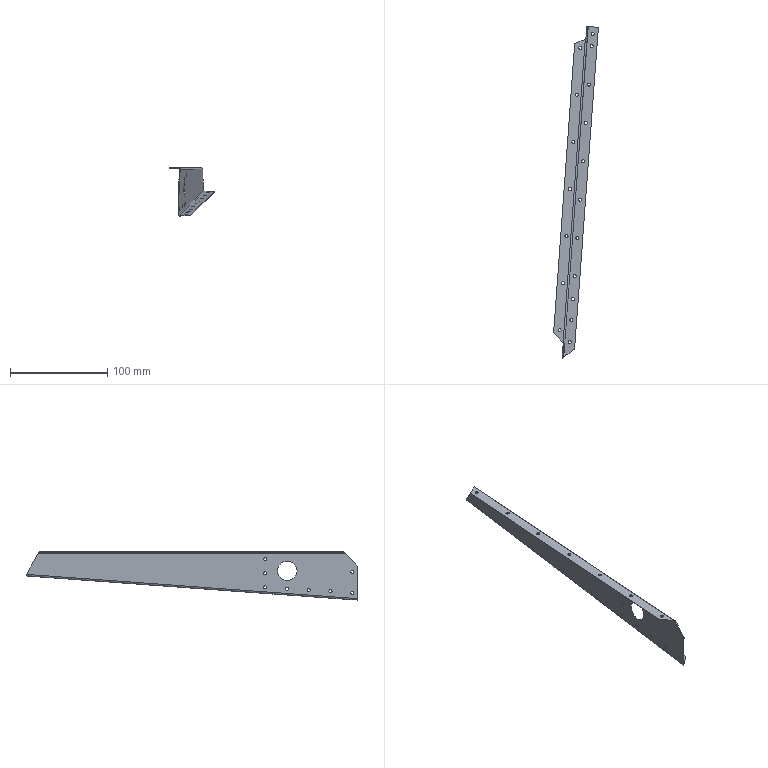Part | SolidWorks | features BaseBody 1 | 1 solid | 81 faces | box 46.078 x 341.712 x 49.508 mm | volume 9487 mm3 | cylinder 60 | plane 15 | spline 6 | commonest cylinder face diameters 3.2 x52 2 x3 3 x3 20 x2